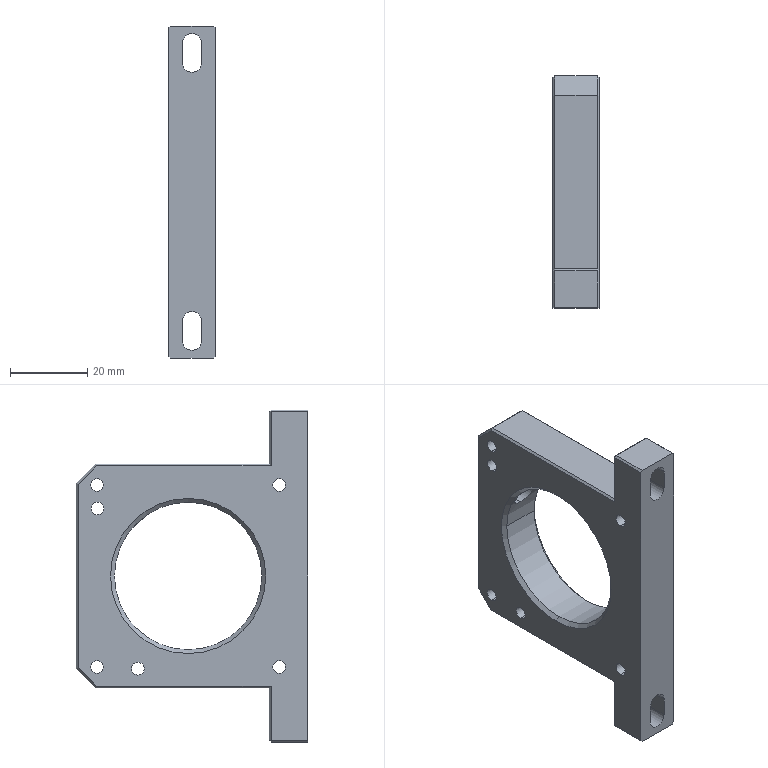Part | NX | features BREP 1 | 1 solid | 66 faces | box 12 x 60 x 86 mm | volume 28967 mm3 | plane 40 | cylinder 22 | cone 4 | commonest cylinder face diameters 3.3 x12 5 x6 6.5 x2 38.2 x2